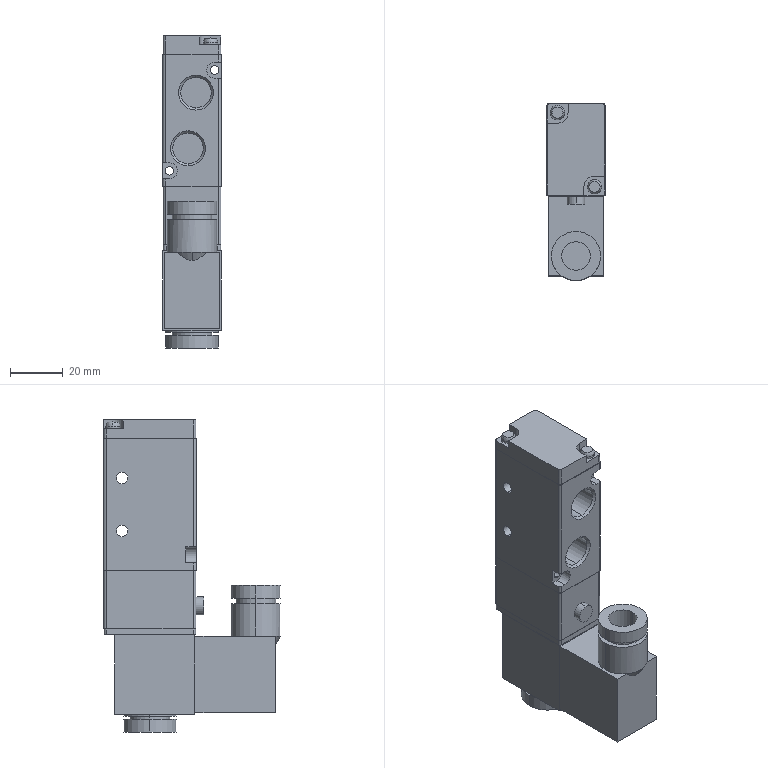Part | SolidWorks | features BaseBody 1 | 1 solid | 137 faces | box 22 x 66.8 x 117.8 mm | volume 99951 mm3 | plane 61 | cylinder 60 | cone 12 | sphere 4 | commonest cylinder face diameters 2 x18 11.445 x6 3.2 x4 4.3 x4 5.4 x4 8.566 x4